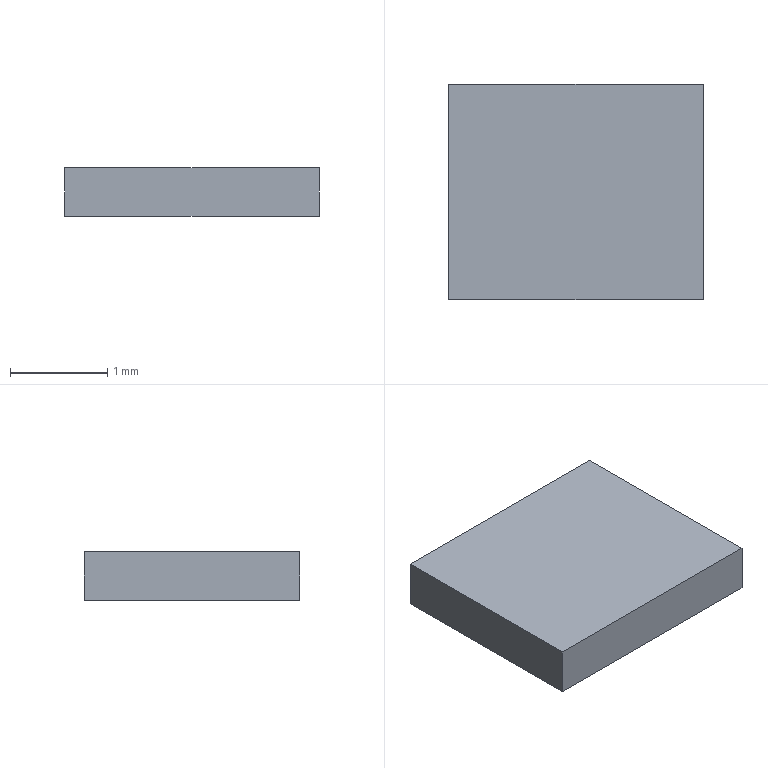Part | Creo | 1 solid | 6 faces | box 2.614 x 2.213 x 0.5 mm | volume 2.892 mm3 | plane 6
STEP:
#1=CARTESIAN_POINT('',(0.,0.,0.));
#2=DIRECTION('',(0.,0.,1.));
#3=DIRECTION('',(1.,0.,0.));
#4=AXIS2_PLACEMENT_3D('',#1,#2,#3);
#5=CARTESIAN_POINT('',(-1.413,-1.214,0.));
#6=VERTEX_POINT('',#5);
#7=CARTESIAN_POINT('',(1.2,-1.214,0.));
#8=VERTEX_POINT('',#7);
#9=CARTESIAN_POINT('',(-1.413,-1.214,0.));
#10=DIRECTION('',(1.,0.,0.));
#11=VECTOR('',#10,2.614);
#12=LINE('',#9,#11);
#13=EDGE_CURVE('',#6,#8,#12,.T.);
#14=ORIENTED_EDGE('',*,*,#13,.T.);
#15=CARTESIAN_POINT('',(1.2,1.,0.));
#16=VERTEX_POINT('',#15);
#17=CARTESIAN_POINT('',(1.2,-1.214,0.));
#18=DIRECTION('',(0.,1.,0.));
#19=VECTOR('',#18,2.213);
#20=LINE('',#17,#19);
#21=EDGE_CURVE('',#8,#16,#20,.T.);
#22=ORIENTED_EDGE('',*,*,#21,.T.);
#23=CARTESIAN_POINT('',(-1.413,1.,0.));
#24=VERTEX_POINT('',#23);
#25=CARTESIAN_POINT('',(1.2,1.,0.));
#26=DIRECTION('',(-1.,0.,0.));
#27=VECTOR('',#26,2.614);
#28=LINE('',#25,#27);
#29=EDGE_CURVE('',#16,#24,#28,.T.);
#30=ORIENTED_EDGE('',*,*,#29,.T.);
#31=CARTESIAN_POINT('',(-1.413,1.,0.));
#32=DIRECTION('',(0.,-1.,0.));
#33=VECTOR('',#32,2.213);
#34=LINE('',#31,#33);
#35=EDGE_CURVE('',#24,#6,#34,.T.);
#36=ORIENTED_EDGE('',*,*,#35,.T.);
#37=EDGE_LOOP('',(#14,#22,#30,#36));
#38=FACE_OUTER_BOUND('',#37,.F.);
#39=CARTESIAN_POINT('',(0.,0.,0.));
#40=DIRECTION('',(0.,0.,1.));
#41=DIRECTION('',(1.,0.,0.));
#42=AXIS2_PLACEMENT_3D('',#39,#40,#41);
#43=PLANE('',#42);
#44=ADVANCED_FACE('',(#38),#43,.F.);
#45=ORIENTED_EDGE('',*,*,#13,.F.);
#46=CARTESIAN_POINT('',(-1.413,-1.214,0.5));
#47=VERTEX_POINT('',#46);
#48=CARTESIAN_POINT('',(-1.413,-1.214,0.));
#49=DIRECTION('',(0.,0.,1.));
#50=VECTOR('',#49,0.5);
#51=LINE('',#48,#50);
#52=EDGE_CURVE('',#6,#47,#51,.T.);
#53=ORIENTED_EDGE('',*,*,#52,.T.);
#54=CARTESIAN_POINT('',(1.2,-1.214,0.5));
#55=VERTEX_POINT('',#54);
#56=CARTESIAN_POINT('',(-1.413,-1.214,0.5));
#57=DIRECTION('',(1.,0.,0.));
#58=VECTOR('',#57,2.614);
#59=LINE('',#56,#58);
#60=EDGE_CURVE('',#47,#55,#59,.T.);
#61=ORIENTED_EDGE('',*,*,#60,.T.);
#62=CARTESIAN_POINT('',(1.2,-1.214,0.));
#63=DIRECTION('',(0.,0.,1.));
#64=VECTOR('',#63,0.5);
#65=LINE('',#62,#64);
#66=EDGE_CURVE('',#8,#55,#65,.T.);
#67=ORIENTED_EDGE('',*,*,#66,.F.);
#68=EDGE_LOOP('',(#45,#53,#61,#67));
#69=FACE_OUTER_BOUND('',#68,.F.);
#70=CARTESIAN_POINT('',(-1.413,-1.214,0.));
#71=DIRECTION('',(0.,-1.,0.));
#72=DIRECTION('',(1.,0.,0.));
#73=AXIS2_PLACEMENT_3D('',#70,#71,#72);
#74=PLANE('',#73);
#75=ADVANCED_FACE('',(#69),#74,.T.);
#76=ORIENTED_EDGE('',*,*,#35,.F.);
#77=CARTESIAN_POINT('',(-1.413,1.,0.5));
#78=VERTEX_POINT('',#77);
#79=CARTESIAN_POINT('',(-1.413,1.,0.));
#80=DIRECTION('',(0.,0.,1.));
#81=VECTOR('',#80,0.5);
#82=LINE('',#79,#81);
#83=EDGE_CURVE('',#24,#78,#82,.T.);
#84=ORIENTED_EDGE('',*,*,#83,.T.);
#85=CARTESIAN_POINT('',(-1.413,1.,0.5));
#86=DIRECTION('',(0.,-1.,0.));
#87=VECTOR('',#86,2.213);
#88=LINE('',#85,#87);
#89=EDGE_CURVE('',#78,#47,#88,.T.);
#90=ORIENTED_EDGE('',*,*,#89,.T.);
#91=ORIENTED_EDGE('',*,*,#52,.F.);
#92=EDGE_LOOP('',(#76,#84,#90,#91));
#93=FACE_OUTER_BOUND('',#92,.F.);
#94=CARTESIAN_POINT('',(-1.413,1.,0.));
#95=DIRECTION('',(-1.,0.,0.));
#96=DIRECTION('',(0.,-1.,0.));
#97=AXIS2_PLACEMENT_3D('',#94,#95,#96);
#98=PLANE('',#97);
#99=ADVANCED_FACE('',(#93),#98,.T.);
#100=ORIENTED_EDGE('',*,*,#29,.F.);
#101=CARTESIAN_POINT('',(1.2,1.,0.5));
#102=VERTEX_POINT('',#101);
#103=CARTESIAN_POINT('',(1.2,1.,0.));
#104=DIRECTION('',(0.,0.,1.));
#105=VECTOR('',#104,0.5);
#106=LINE('',#103,#105);
#107=EDGE_CURVE('',#16,#102,#106,.T.);
#108=ORIENTED_EDGE('',*,*,#107,.T.);
#109=CARTESIAN_POINT('',(1.2,1.,0.5));
#110=DIRECTION('',(-1.,0.,0.));
#111=VECTOR('',#110,2.614);
#112=LINE('',#109,#111);
#113=EDGE_CURVE('',#102,#78,#112,.T.);
#114=ORIENTED_EDGE('',*,*,#113,.T.);
#115=ORIENTED_EDGE('',*,*,#83,.F.);
#116=EDGE_LOOP('',(#100,#108,#114,#115));
#117=FACE_OUTER_BOUND('',#116,.F.);
#118=CARTESIAN_POINT('',(1.2,1.,0.));
#119=DIRECTION('',(0.,1.,0.));
#120=DIRECTION('',(-1.,0.,0.));
#121=AXIS2_PLACEMENT_3D('',#118,#119,#120);
#122=PLANE('',#121);
#123=ADVANCED_FACE('',(#117),#122,.T.);
#124=ORIENTED_EDGE('',*,*,#21,.F.);
#125=ORIENTED_EDGE('',*,*,#66,.T.);
#126=CARTESIAN_POINT('',(1.2,-1.214,0.5));
#127=DIRECTION('',(0.,1.,0.));
#128=VECTOR('',#127,2.213);
#129=LINE('',#126,#128);
#130=EDGE_CURVE('',#55,#102,#129,.T.);
#131=ORIENTED_EDGE('',*,*,#130,.T.);
#132=ORIENTED_EDGE('',*,*,#107,.F.);
#133=EDGE_LOOP('',(#124,#125,#131,#132));
#134=FACE_OUTER_BOUND('',#133,.F.);
#135=CARTESIAN_POINT('',(1.2,-1.214,0.));
#136=DIRECTION('',(1.,0.,0.));
#137=DIRECTION('',(0.,1.,0.));
#138=AXIS2_PLACEMENT_3D('',#135,#136,#137);
#139=PLANE('',#138);
#140=ADVANCED_FACE('',(#134),#139,.T.);
#141=ORIENTED_EDGE('',*,*,#60,.F.);
#142=ORIENTED_EDGE('',*,*,#89,.F.);
#143=ORIENTED_EDGE('',*,*,#113,.F.);
#144=ORIENTED_EDGE('',*,*,#130,.F.);
#145=EDGE_LOOP('',(#141,#142,#143,#144));
#146=FACE_OUTER_BOUND('',#145,.F.);
#147=CARTESIAN_POINT('',(0.,0.,0.5));
#148=DIRECTION('',(0.,0.,1.));
#149=DIRECTION('',(1.,0.,0.));
#150=AXIS2_PLACEMENT_3D('',#147,#148,#149);
#151=PLANE('',#150);
#152=ADVANCED_FACE('',(#146),#151,.T.);
#153=CLOSED_SHELL('',(#44,#75,#99,#123,#140,#152));
#154=MANIFOLD_SOLID_BREP('',#153);
#155=(LENGTH_UNIT()NAMED_UNIT(*)SI_UNIT(.MILLI.,.METRE.));
#156=UNCERTAINTY_MEASURE_WITH_UNIT(LENGTH_MEASURE(0.0003461),#155,'','');
#157=(NAMED_UNIT(*)PLANE_ANGLE_UNIT()SI_UNIT($,.RADIAN.));
#158=PLANE_ANGLE_MEASURE_WITH_UNIT(PLANE_ANGLE_MEASURE(0.01745),#157);
#159=(CONVERSION_BASED_UNIT('DEGREE',#158)NAMED_UNIT(*)PLANE_ANGLE_UNIT());
#160=(NAMED_UNIT(*)SI_UNIT($,.STERADIAN.)SOLID_ANGLE_UNIT());
#161=(GEOMETRIC_REPRESENTATION_CONTEXT(3)GLOBAL_UNCERTAINTY_ASSIGNED_CONTEXT((#156))GLOBAL_UNIT_ASSIGNED_CONTEXT((#155,#159,#160))REPRESENTATION_CONTEXT('',''));
#162=ADVANCED_BREP_SHAPE_REPRESENTATION('',(#4,#154),#161);